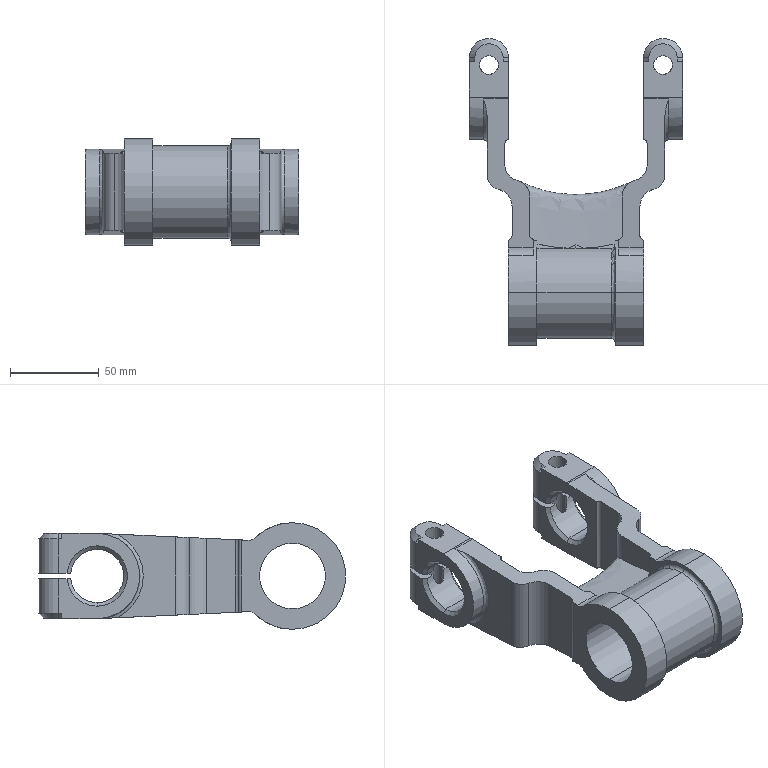Part | NX | features DATUM_PLANE 8, DELETE FACE 6, DATUM_CSYS 4, SKETCH 3, TRIM BODY 3, CHAMFER 2, SPLIT BODY 2, UNITE 2, BLEND 1, BREP 1, Delete Body 1, EXTRUDE 1, MOVE_FACE 1, REPLACE_FACE 1, SKIN 1 | 1 solid | 138 faces | box 120 x 173 x 60 mm | volume 247159 mm3 | cylinder 57 | plane 50 | cone 16 | spline 10 | torus 5 | commonest cylinder face diameters 4 x12 10.5 x8 12 x6 30 x6 60 x6 16 x4